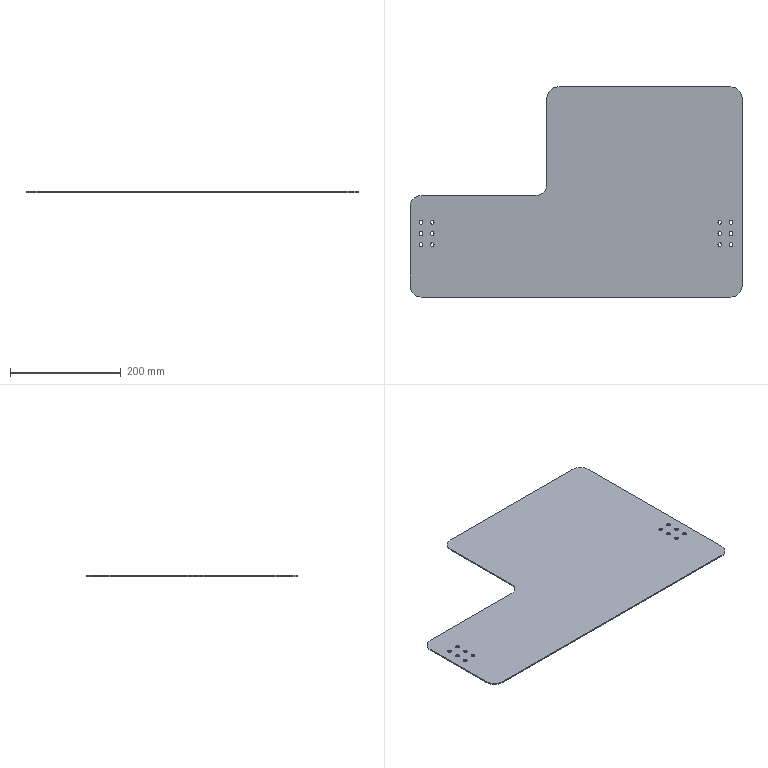Part | STEP file | MT-COMBO-119-S010 | 1 solid | 38 faces | box 600 x 380 x 2 mm | volume 357256 mm3 | cylinder 30 | plane 8 | commonest cylinder face diameters 6.8 x24 40 x6
STEP:
#1=CARTESIAN_POINT('',(-263.4,-15.,2.));
#2=VERTEX_POINT('',#1);
#3=CARTESIAN_POINT('',(-256.6,-15.,2.));
#4=VERTEX_POINT('',#3);
#5=CARTESIAN_POINT('',(-260.,-15.,2.));
#6=DIRECTION('',(0.,0.,1.));
#7=DIRECTION('',(1.,0.,0.));
#8=AXIS2_PLACEMENT_3D('',#5,#6,#7);
#9=CIRCLE('',#8,3.4);
#10=EDGE_CURVE('',#2,#4,#9,.T.);
#11=ORIENTED_EDGE('',*,*,#10,.T.);
#12=CARTESIAN_POINT('',(-256.6,-15.,0.));
#13=VERTEX_POINT('',#12);
#14=CARTESIAN_POINT('',(-256.6,-15.,0.));
#15=DIRECTION('',(0.,0.,-1.));
#16=VECTOR('',#15,1000.);
#17=LINE('',#14,#16);
#18=EDGE_CURVE('',#4,#13,#17,.T.);
#19=ORIENTED_EDGE('',*,*,#18,.T.);
#20=CARTESIAN_POINT('',(-263.4,-15.,0.));
#21=VERTEX_POINT('',#20);
#22=CARTESIAN_POINT('',(-260.,-15.,0.));
#23=DIRECTION('',(0.,0.,-1.));
#24=DIRECTION('',(-1.,0.,0.));
#25=AXIS2_PLACEMENT_3D('',#22,#23,#24);
#26=CIRCLE('',#25,3.4);
#27=EDGE_CURVE('',#13,#21,#26,.T.);
#28=ORIENTED_EDGE('',*,*,#27,.T.);
#29=CARTESIAN_POINT('',(-263.4,-15.,0.));
#30=DIRECTION('',(0.,0.,-1.));
#31=VECTOR('',#30,1000.);
#32=LINE('',#29,#31);
#33=EDGE_CURVE('',#2,#21,#32,.T.);
#34=ORIENTED_EDGE('',*,*,#33,.F.);
#35=EDGE_LOOP('',(#11,#19,#28,#34));
#36=FACE_OUTER_BOUND('',#35,.T.);
#37=CARTESIAN_POINT('',(-260.,-15.,0.));
#38=DIRECTION('',(0.,0.,-1.));
#39=DIRECTION('',(-1.,0.,0.));
#40=AXIS2_PLACEMENT_3D('',#37,#38,#39);
#41=CYLINDRICAL_SURFACE('',#40,3.4);
#42=ADVANCED_FACE('',(#36),#41,.F.);
#43=CARTESIAN_POINT('',(-283.4,-15.,2.));
#44=VERTEX_POINT('',#43);
#45=CARTESIAN_POINT('',(-276.6,-15.,2.));
#46=VERTEX_POINT('',#45);
#47=CARTESIAN_POINT('',(-280.,-15.,2.));
#48=DIRECTION('',(0.,0.,1.));
#49=DIRECTION('',(1.,0.,0.));
#50=AXIS2_PLACEMENT_3D('',#47,#48,#49);
#51=CIRCLE('',#50,3.4);
#52=EDGE_CURVE('',#44,#46,#51,.T.);
#53=ORIENTED_EDGE('',*,*,#52,.T.);
#54=CARTESIAN_POINT('',(-276.6,-15.,0.));
#55=VERTEX_POINT('',#54);
#56=CARTESIAN_POINT('',(-276.6,-15.,0.));
#57=DIRECTION('',(0.,0.,-1.));
#58=VECTOR('',#57,1000.);
#59=LINE('',#56,#58);
#60=EDGE_CURVE('',#46,#55,#59,.T.);
#61=ORIENTED_EDGE('',*,*,#60,.T.);
#62=CARTESIAN_POINT('',(-283.4,-15.,0.));
#63=VERTEX_POINT('',#62);
#64=CARTESIAN_POINT('',(-280.,-15.,0.));
#65=DIRECTION('',(0.,0.,-1.));
#66=DIRECTION('',(-1.,0.,0.));
#67=AXIS2_PLACEMENT_3D('',#64,#65,#66);
#68=CIRCLE('',#67,3.4);
#69=EDGE_CURVE('',#55,#63,#68,.T.);
#70=ORIENTED_EDGE('',*,*,#69,.T.);
#71=CARTESIAN_POINT('',(-283.4,-15.,0.));
#72=DIRECTION('',(0.,0.,-1.));
#73=VECTOR('',#72,1000.);
#74=LINE('',#71,#73);
#75=EDGE_CURVE('',#44,#63,#74,.T.);
#76=ORIENTED_EDGE('',*,*,#75,.F.);
#77=EDGE_LOOP('',(#53,#61,#70,#76));
#78=FACE_OUTER_BOUND('',#77,.T.);
#79=CARTESIAN_POINT('',(-280.,-15.,0.));
#80=DIRECTION('',(0.,0.,-1.));
#81=DIRECTION('',(-1.,0.,0.));
#82=AXIS2_PLACEMENT_3D('',#79,#80,#81);
#83=CYLINDRICAL_SURFACE('',#82,3.4);
#84=ADVANCED_FACE('',(#78),#83,.F.);
#85=CARTESIAN_POINT('',(-263.4,-35.,2.));
#86=VERTEX_POINT('',#85);
#87=CARTESIAN_POINT('',(-256.6,-35.,2.));
#88=VERTEX_POINT('',#87);
#89=CARTESIAN_POINT('',(-260.,-35.,2.));
#90=DIRECTION('',(0.,0.,1.));
#91=DIRECTION('',(1.,0.,0.));
#92=AXIS2_PLACEMENT_3D('',#89,#90,#91);
#93=CIRCLE('',#92,3.4);
#94=EDGE_CURVE('',#86,#88,#93,.T.);
#95=ORIENTED_EDGE('',*,*,#94,.T.);
#96=CARTESIAN_POINT('',(-256.6,-35.,0.));
#97=VERTEX_POINT('',#96);
#98=CARTESIAN_POINT('',(-256.6,-35.,0.));
#99=DIRECTION('',(0.,0.,-1.));
#100=VECTOR('',#99,1000.);
#101=LINE('',#98,#100);
#102=EDGE_CURVE('',#88,#97,#101,.T.);
#103=ORIENTED_EDGE('',*,*,#102,.T.);
#104=CARTESIAN_POINT('',(-263.4,-35.,0.));
#105=VERTEX_POINT('',#104);
#106=CARTESIAN_POINT('',(-260.,-35.,0.));
#107=DIRECTION('',(0.,0.,-1.));
#108=DIRECTION('',(-1.,0.,0.));
#109=AXIS2_PLACEMENT_3D('',#106,#107,#108);
#110=CIRCLE('',#109,3.4);
#111=EDGE_CURVE('',#97,#105,#110,.T.);
#112=ORIENTED_EDGE('',*,*,#111,.T.);
#113=CARTESIAN_POINT('',(-263.4,-35.,0.));
#114=DIRECTION('',(0.,0.,-1.));
#115=VECTOR('',#114,1000.);
#116=LINE('',#113,#115);
#117=EDGE_CURVE('',#86,#105,#116,.T.);
#118=ORIENTED_EDGE('',*,*,#117,.F.);
#119=EDGE_LOOP('',(#95,#103,#112,#118));
#120=FACE_OUTER_BOUND('',#119,.T.);
#121=CARTESIAN_POINT('',(-260.,-35.,0.));
#122=DIRECTION('',(0.,0.,-1.));
#123=DIRECTION('',(-1.,0.,0.));
#124=AXIS2_PLACEMENT_3D('',#121,#122,#123);
#125=CYLINDRICAL_SURFACE('',#124,3.4);
#126=ADVANCED_FACE('',(#120),#125,.F.);
#127=CARTESIAN_POINT('',(-283.4,-35.,2.));
#128=VERTEX_POINT('',#127);
#129=CARTESIAN_POINT('',(-276.6,-35.,2.));
#130=VERTEX_POINT('',#129);
#131=CARTESIAN_POINT('',(-280.,-35.,2.));
#132=DIRECTION('',(0.,0.,1.));
#133=DIRECTION('',(1.,0.,0.));
#134=AXIS2_PLACEMENT_3D('',#131,#132,#133);
#135=CIRCLE('',#134,3.4);
#136=EDGE_CURVE('',#128,#130,#135,.T.);
#137=ORIENTED_EDGE('',*,*,#136,.T.);
#138=CARTESIAN_POINT('',(-276.6,-35.,0.));
#139=VERTEX_POINT('',#138);
#140=CARTESIAN_POINT('',(-276.6,-35.,0.));
#141=DIRECTION('',(0.,0.,-1.));
#142=VECTOR('',#141,1000.);
#143=LINE('',#140,#142);
#144=EDGE_CURVE('',#130,#139,#143,.T.);
#145=ORIENTED_EDGE('',*,*,#144,.T.);
#146=CARTESIAN_POINT('',(-283.4,-35.,0.));
#147=VERTEX_POINT('',#146);
#148=CARTESIAN_POINT('',(-280.,-35.,0.));
#149=DIRECTION('',(0.,0.,-1.));
#150=DIRECTION('',(-1.,0.,0.));
#151=AXIS2_PLACEMENT_3D('',#148,#149,#150);
#152=CIRCLE('',#151,3.4);
#153=EDGE_CURVE('',#139,#147,#152,.T.);
#154=ORIENTED_EDGE('',*,*,#153,.T.);
#155=CARTESIAN_POINT('',(-283.4,-35.,0.));
#156=DIRECTION('',(0.,0.,-1.));
#157=VECTOR('',#156,1000.);
#158=LINE('',#155,#157);
#159=EDGE_CURVE('',#128,#147,#158,.T.);
#160=ORIENTED_EDGE('',*,*,#159,.F.);
#161=EDGE_LOOP('',(#137,#145,#154,#160));
#162=FACE_OUTER_BOUND('',#161,.T.);
#163=CARTESIAN_POINT('',(-280.,-35.,0.));
#164=DIRECTION('',(0.,0.,-1.));
#165=DIRECTION('',(-1.,0.,0.));
#166=AXIS2_PLACEMENT_3D('',#163,#164,#165);
#167=CYLINDRICAL_SURFACE('',#166,3.4);
#168=ADVANCED_FACE('',(#162),#167,.F.);
#169=CARTESIAN_POINT('',(-283.4,-55.,2.));
#170=VERTEX_POINT('',#169);
#171=CARTESIAN_POINT('',(-276.6,-55.,2.));
#172=VERTEX_POINT('',#171);
#173=CARTESIAN_POINT('',(-280.,-55.,2.));
#174=DIRECTION('',(0.,0.,1.));
#175=DIRECTION('',(1.,0.,0.));
#176=AXIS2_PLACEMENT_3D('',#173,#174,#175);
#177=CIRCLE('',#176,3.4);
#178=EDGE_CURVE('',#170,#172,#177,.T.);
#179=ORIENTED_EDGE('',*,*,#178,.T.);
#180=CARTESIAN_POINT('',(-276.6,-55.,0.));
#181=VERTEX_POINT('',#180);
#182=CARTESIAN_POINT('',(-276.6,-55.,0.));
#183=DIRECTION('',(0.,0.,-1.));
#184=VECTOR('',#183,1000.);
#185=LINE('',#182,#184);
#186=EDGE_CURVE('',#172,#181,#185,.T.);
#187=ORIENTED_EDGE('',*,*,#186,.T.);
#188=CARTESIAN_POINT('',(-283.4,-55.,0.));
#189=VERTEX_POINT('',#188);
#190=CARTESIAN_POINT('',(-280.,-55.,0.));
#191=DIRECTION('',(0.,0.,-1.));
#192=DIRECTION('',(-1.,0.,0.));
#193=AXIS2_PLACEMENT_3D('',#190,#191,#192);
#194=CIRCLE('',#193,3.4);
#195=EDGE_CURVE('',#181,#189,#194,.T.);
#196=ORIENTED_EDGE('',*,*,#195,.T.);
#197=CARTESIAN_POINT('',(-283.4,-55.,0.));
#198=DIRECTION('',(0.,0.,-1.));
#199=VECTOR('',#198,1000.);
#200=LINE('',#197,#199);
#201=EDGE_CURVE('',#170,#189,#200,.T.);
#202=ORIENTED_EDGE('',*,*,#201,.F.);
#203=EDGE_LOOP('',(#179,#187,#196,#202));
#204=FACE_OUTER_BOUND('',#203,.T.);
#205=CARTESIAN_POINT('',(-280.,-55.,0.));
#206=DIRECTION('',(0.,0.,-1.));
#207=DIRECTION('',(-1.,0.,0.));
#208=AXIS2_PLACEMENT_3D('',#205,#206,#207);
#209=CYLINDRICAL_SURFACE('',#208,3.4);
#210=ADVANCED_FACE('',(#204),#209,.F.);
#211=CARTESIAN_POINT('',(-263.4,-55.,2.));
#212=VERTEX_POINT('',#211);
#213=CARTESIAN_POINT('',(-256.6,-55.,2.));
#214=VERTEX_POINT('',#213);
#215=CARTESIAN_POINT('',(-260.,-55.,2.));
#216=DIRECTION('',(0.,0.,1.));
#217=DIRECTION('',(1.,0.,0.));
#218=AXIS2_PLACEMENT_3D('',#215,#216,#217);
#219=CIRCLE('',#218,3.4);
#220=EDGE_CURVE('',#212,#214,#219,.T.);
#221=ORIENTED_EDGE('',*,*,#220,.T.);
#222=CARTESIAN_POINT('',(-256.6,-55.,0.));
#223=VERTEX_POINT('',#222);
#224=CARTESIAN_POINT('',(-256.6,-55.,0.));
#225=DIRECTION('',(0.,0.,-1.));
#226=VECTOR('',#225,1000.);
#227=LINE('',#224,#226);
#228=EDGE_CURVE('',#214,#223,#227,.T.);
#229=ORIENTED_EDGE('',*,*,#228,.T.);
#230=CARTESIAN_POINT('',(-263.4,-55.,0.));
#231=VERTEX_POINT('',#230);
#232=CARTESIAN_POINT('',(-260.,-55.,0.));
#233=DIRECTION('',(0.,0.,-1.));
#234=DIRECTION('',(-1.,0.,0.));
#235=AXIS2_PLACEMENT_3D('',#232,#233,#234);
#236=CIRCLE('',#235,3.4);
#237=EDGE_CURVE('',#223,#231,#236,.T.);
#238=ORIENTED_EDGE('',*,*,#237,.T.);
#239=CARTESIAN_POINT('',(-263.4,-55.,0.));
#240=DIRECTION('',(0.,0.,-1.));
#241=VECTOR('',#240,1000.);
#242=LINE('',#239,#241);
#243=EDGE_CURVE('',#212,#231,#242,.T.);
#244=ORIENTED_EDGE('',*,*,#243,.F.);
#245=EDGE_LOOP('',(#221,#229,#238,#244));
#246=FACE_OUTER_BOUND('',#245,.T.);
#247=CARTESIAN_POINT('',(-260.,-55.,0.));
#248=DIRECTION('',(0.,0.,-1.));
#249=DIRECTION('',(-1.,0.,0.));
#250=AXIS2_PLACEMENT_3D('',#247,#248,#249);
#251=CYLINDRICAL_SURFACE('',#250,3.4);
#252=ADVANCED_FACE('',(#246),#251,.F.);
#253=CARTESIAN_POINT('',(256.6,-15.,2.));
#254=VERTEX_POINT('',#253);
#255=CARTESIAN_POINT('',(263.4,-15.,2.));
#256=VERTEX_POINT('',#255);
#257=CARTESIAN_POINT('',(260.,-15.,2.));
#258=DIRECTION('',(0.,0.,1.));
#259=DIRECTION('',(1.,0.,0.));
#260=AXIS2_PLACEMENT_3D('',#257,#258,#259);
#261=CIRCLE('',#260,3.4);
#262=EDGE_CURVE('',#254,#256,#261,.T.);
#263=ORIENTED_EDGE('',*,*,#262,.T.);
#264=CARTESIAN_POINT('',(263.4,-15.,0.));
#265=VERTEX_POINT('',#264);
#266=CARTESIAN_POINT('',(263.4,-15.,0.));
#267=DIRECTION('',(0.,0.,-1.));
#268=VECTOR('',#267,1000.);
#269=LINE('',#266,#268);
#270=EDGE_CURVE('',#256,#265,#269,.T.);
#271=ORIENTED_EDGE('',*,*,#270,.T.);
#272=CARTESIAN_POINT('',(256.6,-15.,0.));
#273=VERTEX_POINT('',#272);
#274=CARTESIAN_POINT('',(260.,-15.,0.));
#275=DIRECTION('',(0.,0.,-1.));
#276=DIRECTION('',(-1.,0.,0.));
#277=AXIS2_PLACEMENT_3D('',#274,#275,#276);
#278=CIRCLE('',#277,3.4);
#279=EDGE_CURVE('',#265,#273,#278,.T.);
#280=ORIENTED_EDGE('',*,*,#279,.T.);
#281=CARTESIAN_POINT('',(256.6,-15.,0.));
#282=DIRECTION('',(0.,0.,-1.));
#283=VECTOR('',#282,1000.);
#284=LINE('',#281,#283);
#285=EDGE_CURVE('',#254,#273,#284,.T.);
#286=ORIENTED_EDGE('',*,*,#285,.F.);
#287=EDGE_LOOP('',(#263,#271,#280,#286));
#288=FACE_OUTER_BOUND('',#287,.T.);
#289=CARTESIAN_POINT('',(260.,-15.,0.));
#290=DIRECTION('',(0.,0.,-1.));
#291=DIRECTION('',(-1.,0.,0.));
#292=AXIS2_PLACEMENT_3D('',#289,#290,#291);
#293=CYLINDRICAL_SURFACE('',#292,3.4);
#294=ADVANCED_FACE('',(#288),#293,.F.);
#295=CARTESIAN_POINT('',(276.6,-15.,2.));
#296=VERTEX_POINT('',#295);
#297=CARTESIAN_POINT('',(283.4,-15.,2.));
#298=VERTEX_POINT('',#297);
#299=CARTESIAN_POINT('',(280.,-15.,2.));
#300=DIRECTION('',(0.,0.,1.));
#301=DIRECTION('',(1.,0.,0.));
#302=AXIS2_PLACEMENT_3D('',#299,#300,#301);
#303=CIRCLE('',#302,3.4);
#304=EDGE_CURVE('',#296,#298,#303,.T.);
#305=ORIENTED_EDGE('',*,*,#304,.T.);
#306=CARTESIAN_POINT('',(283.4,-15.,0.));
#307=VERTEX_POINT('',#306);
#308=CARTESIAN_POINT('',(283.4,-15.,0.));
#309=DIRECTION('',(0.,0.,-1.));
#310=VECTOR('',#309,1000.);
#311=LINE('',#308,#310);
#312=EDGE_CURVE('',#298,#307,#311,.T.);
#313=ORIENTED_EDGE('',*,*,#312,.T.);
#314=CARTESIAN_POINT('',(276.6,-15.,0.));
#315=VERTEX_POINT('',#314);
#316=CARTESIAN_POINT('',(280.,-15.,0.));
#317=DIRECTION('',(0.,0.,-1.));
#318=DIRECTION('',(-1.,0.,0.));
#319=AXIS2_PLACEMENT_3D('',#316,#317,#318);
#320=CIRCLE('',#319,3.4);
#321=EDGE_CURVE('',#307,#315,#320,.T.);
#322=ORIENTED_EDGE('',*,*,#321,.T.);
#323=CARTESIAN_POINT('',(276.6,-15.,0.));
#324=DIRECTION('',(0.,0.,-1.));
#325=VECTOR('',#324,1000.);
#326=LINE('',#323,#325);
#327=EDGE_CURVE('',#296,#315,#326,.T.);
#328=ORIENTED_EDGE('',*,*,#327,.F.);
#329=EDGE_LOOP('',(#305,#313,#322,#328));
#330=FACE_OUTER_BOUND('',#329,.T.);
#331=CARTESIAN_POINT('',(280.,-15.,0.));
#332=DIRECTION('',(0.,0.,-1.));
#333=DIRECTION('',(-1.,0.,0.));
#334=AXIS2_PLACEMENT_3D('',#331,#332,#333);
#335=CYLINDRICAL_SURFACE('',#334,3.4);
#336=ADVANCED_FACE('',(#330),#335,.F.);
#337=CARTESIAN_POINT('',(256.6,-35.,2.));
#338=VERTEX_POINT('',#337);
#339=CARTESIAN_POINT('',(263.4,-35.,2.));
#340=VERTEX_POINT('',#339);
#341=CARTESIAN_POINT('',(260.,-35.,2.));
#342=DIRECTION('',(0.,0.,1.));
#343=DIRECTION('',(1.,0.,0.));
#344=AXIS2_PLACEMENT_3D('',#341,#342,#343);
#345=CIRCLE('',#344,3.4);
#346=EDGE_CURVE('',#338,#340,#345,.T.);
#347=ORIENTED_EDGE('',*,*,#346,.T.);
#348=CARTESIAN_POINT('',(263.4,-35.,0.));
#349=VERTEX_POINT('',#348);
#350=CARTESIAN_POINT('',(263.4,-35.,0.));
#351=DIRECTION('',(0.,0.,-1.));
#352=VECTOR('',#351,1000.);
#353=LINE('',#350,#352);
#354=EDGE_CURVE('',#340,#349,#353,.T.);
#355=ORIENTED_EDGE('',*,*,#354,.T.);
#356=CARTESIAN_POINT('',(256.6,-35.,0.));
#357=VERTEX_POINT('',#356);
#358=CARTESIAN_POINT('',(260.,-35.,0.));
#359=DIRECTION('',(0.,0.,-1.));
#360=DIRECTION('',(-1.,0.,0.));
#361=AXIS2_PLACEMENT_3D('',#358,#359,#360);
#362=CIRCLE('',#361,3.4);
#363=EDGE_CURVE('',#349,#357,#362,.T.);
#364=ORIENTED_EDGE('',*,*,#363,.T.);
#365=CARTESIAN_POINT('',(256.6,-35.,0.));
#366=DIRECTION('',(0.,0.,-1.));
#367=VECTOR('',#366,1000.);
#368=LINE('',#365,#367);
#369=EDGE_CURVE('',#338,#357,#368,.T.);
#370=ORIENTED_EDGE('',*,*,#369,.F.);
#371=EDGE_LOOP('',(#347,#355,#364,#370));
#372=FACE_OUTER_BOUND('',#371,.T.);
#373=CARTESIAN_POINT('',(260.,-35.,0.));
#374=DIRECTION('',(0.,0.,-1.));
#375=DIRECTION('',(-1.,0.,0.));
#376=AXIS2_PLACEMENT_3D('',#373,#374,#375);
#377=CYLINDRICAL_SURFACE('',#376,3.4);
#378=ADVANCED_FACE('',(#372),#377,.F.);
#379=CARTESIAN_POINT('',(276.6,-35.,2.));
#380=VERTEX_POINT('',#379);
#381=CARTESIAN_POINT('',(283.4,-35.,2.));
#382=VERTEX_POINT('',#381);
#383=CARTESIAN_POINT('',(280.,-35.,2.));
#384=DIRECTION('',(0.,0.,1.));
#385=DIRECTION('',(1.,0.,0.));
#386=AXIS2_PLACEMENT_3D('',#383,#384,#385);
#387=CIRCLE('',#386,3.4);
#388=EDGE_CURVE('',#380,#382,#387,.T.);
#389=ORIENTED_EDGE('',*,*,#388,.T.);
#390=CARTESIAN_POINT('',(283.4,-35.,0.));
#391=VERTEX_POINT('',#390);
#392=CARTESIAN_POINT('',(283.4,-35.,0.));
#393=DIRECTION('',(0.,0.,-1.));
#394=VECTOR('',#393,1000.);
#395=LINE('',#392,#394);
#396=EDGE_CURVE('',#382,#391,#395,.T.);
#397=ORIENTED_EDGE('',*,*,#396,.T.);
#398=CARTESIAN_POINT('',(276.6,-35.,0.));
#399=VERTEX_POINT('',#398);
#400=CARTESIAN_POINT('',(280.,-35.,0.));
#401=DIRECTION('',(0.,0.,-1.));
#402=DIRECTION('',(-1.,0.,0.));
#403=AXIS2_PLACEMENT_3D('',#400,#401,#402);
#404=CIRCLE('',#403,3.4);
#405=EDGE_CURVE('',#391,#399,#404,.T.);
#406=ORIENTED_EDGE('',*,*,#405,.T.);
#407=CARTESIAN_POINT('',(276.6,-35.,0.));
#408=DIRECTION('',(0.,0.,-1.));
#409=VECTOR('',#408,1000.);
#410=LINE('',#407,#409);
#411=EDGE_CURVE('',#380,#399,#410,.T.);
#412=ORIENTED_EDGE('',*,*,#411,.F.);
#413=EDGE_LOOP('',(#389,#397,#406,#412));
#414=FACE_OUTER_BOUND('',#413,.T.);
#415=CARTESIAN_POINT('',(280.,-35.,0.));
#416=DIRECTION('',(0.,0.,-1.));
#417=DIRECTION('',(-1.,0.,0.));
#418=AXIS2_PLACEMENT_3D('',#415,#416,#417);
#419=CYLINDRICAL_SURFACE('',#418,3.4);
#420=ADVANCED_FACE('',(#414),#419,.F.);
#421=CARTESIAN_POINT('',(276.6,-55.,2.));
#422=VERTEX_POINT('',#421);
#423=CARTESIAN_POINT('',(283.4,-55.,2.));
#424=VERTEX_POINT('',#423);
#425=CARTESIAN_POINT('',(280.,-55.,2.));
#426=DIRECTION('',(0.,0.,1.));
#427=DIRECTION('',(1.,0.,0.));
#428=AXIS2_PLACEMENT_3D('',#425,#426,#427);
#429=CIRCLE('',#428,3.4);
#430=EDGE_CURVE('',#422,#424,#429,.T.);
#431=ORIENTED_EDGE('',*,*,#430,.T.);
#432=CARTESIAN_POINT('',(283.4,-55.,0.));
#433=VERTEX_POINT('',#432);
#434=CARTESIAN_POINT('',(283.4,-55.,0.));
#435=DIRECTION('',(0.,0.,-1.));
#436=VECTOR('',#435,1000.);
#437=LINE('',#434,#436);
#438=EDGE_CURVE('',#424,#433,#437,.T.);
#439=ORIENTED_EDGE('',*,*,#438,.T.);
#440=CARTESIAN_POINT('',(276.6,-55.,0.));
#441=VERTEX_POINT('',#440);
#442=CARTESIAN_POINT('',(280.,-55.,0.));
#443=DIRECTION('',(0.,0.,-1.));
#444=DIRECTION('',(-1.,0.,0.));
#445=AXIS2_PLACEMENT_3D('',#442,#443,#444);
#446=CIRCLE('',#445,3.4);
#447=EDGE_CURVE('',#433,#441,#446,.T.);
#448=ORIENTED_EDGE('',*,*,#447,.T.);
#449=CARTESIAN_POINT('',(276.6,-55.,0.));
#450=DIRECTION('',(0.,0.,-1.));
#451=VECTOR('',#450,1000.);
#452=LINE('',#449,#451);
#453=EDGE_CURVE('',#422,#441,#452,.T.);
#454=ORIENTED_EDGE('',*,*,#453,.F.);
#455=EDGE_LOOP('',(#431,#439,#448,#454));
#456=FACE_OUTER_BOUND('',#455,.T.);
#457=CARTESIAN_POINT('',(280.,-55.,0.));
#458=DIRECTION('',(0.,0.,-1.));
#459=DIRECTION('',(-1.,0.,0.));
#460=AXIS2_PLACEMENT_3D('',#457,#458,#459);
#461=CYLINDRICAL_SURFACE('',#460,3.4);
#462=ADVANCED_FACE('',(#456),#461,.F.);
#463=CARTESIAN_POINT('',(256.6,-55.,2.));
#464=VERTEX_POINT('',#463);
#465=CARTESIAN_POINT('',(263.4,-55.,2.));
#466=VERTEX_POINT('',#465);
#467=CARTESIAN_POINT('',(260.,-55.,2.));
#468=DIRECTION('',(0.,0.,1.));
#469=DIRECTION('',(1.,0.,0.));
#470=AXIS2_PLACEMENT_3D('',#467,#468,#469);
#471=CIRCLE('',#470,3.4);
#472=EDGE_CURVE('',#464,#466,#471,.T.);
#473=ORIENTED_EDGE('',*,*,#472,.T.);
#474=CARTESIAN_POINT('',(263.4,-55.,0.));
#475=VERTEX_POINT('',#474);
#476=CARTESIAN_POINT('',(263.4,-55.,0.));
#477=DIRECTION('',(0.,0.,-1.));
#478=VECTOR('',#477,1000.);
#479=LINE('',#476,#478);
#480=EDGE_CURVE('',#466,#475,#479,.T.);
#481=ORIENTED_EDGE('',*,*,#480,.T.);
#482=CARTESIAN_POINT('',(256.6,-55.,0.));
#483=VERTEX_POINT('',#482);
#484=CARTESIAN_POINT('',(260.,-55.,0.));
#485=DIRECTION('',(0.,0.,-1.));
#486=DIRECTION('',(-1.,0.,0.));
#487=AXIS2_PLACEMENT_3D('',#484,#485,#486);
#488=CIRCLE('',#487,3.4);
#489=EDGE_CURVE('',#475,#483,#488,.T.);
#490=ORIENTED_EDGE('',*,*,#489,.T.);
#491=CARTESIAN_POINT('',(256.6,-55.,0.));
#492=DIRECTION('',(0.,0.,-1.));
#493=VECTOR('',#492,1000.);
#494=LINE('',#491,#493);
#495=EDGE_CURVE('',#464,#483,#494,.T.);
#496=ORIENTED_EDGE('',*,*,#495,.F.);
#497=EDGE_LOOP('',(#473,#481,#490,#496));
#498=FACE_OUTER_BOUND('',#497,.T.);
#499=CARTESIAN_POINT('',(260.,-55.,0.));
#500=DIRECTION('',(0.,0.,-1.));
#501=DIRECTION('',(-1.,0.,0.));
#502=AXIS2_PLACEMENT_3D('',#499,#500,#501);
#503=CYLINDRICAL_SURFACE('',#502,3.4);
#504=ADVANCED_FACE('',(#498),#503,.F.);
#505=CARTESIAN_POINT('',(-260.,-15.,0.));
#506=DIRECTION('',(0.,0.,-1.));
#507=DIRECTION('',(-1.,0.,0.));
#508=AXIS2_PLACEMENT_3D('',#505,#506,#507);
#509=CIRCLE('',#508,3.4);
#510=EDGE_CURVE('',#21,#13,#509,.T.);
#511=ORIENTED_EDGE('',*,*,#510,.F.);
#512=ORIENTED_EDGE('',*,*,#27,.F.);
#513=EDGE_LOOP('',(#511,#512));
#514=FACE_BOUND('',#513,.T.);
#515=CARTESIAN_POINT('',(-280.,-15.,0.));
#516=DIRECTION('',(0.,0.,-1.));
#517=DIRECTION('',(-1.,0.,0.));
#518=AXIS2_PLACEMENT_3D('',#515,#516,#517);
#519=CIRCLE('',#518,3.4);
#520=EDGE_CURVE('',#63,#55,#519,.T.);
#521=ORIENTED_EDGE('',*,*,#520,.F.);
#522=ORIENTED_EDGE('',*,*,#69,.F.);
#523=EDGE_LOOP('',(#521,#522));
#524=FACE_BOUND('',#523,.T.);
#525=CARTESIAN_POINT('',(-260.,-35.,0.));
#526=DIRECTION('',(0.,0.,-1.));
#527=DIRECTION('',(-1.,0.,0.));
#528=AXIS2_PLACEMENT_3D('',#525,#526,#527);
#529=CIRCLE('',#528,3.4);
#530=EDGE_CURVE('',#105,#97,#529,.T.);
#531=ORIENTED_EDGE('',*,*,#530,.F.);
#532=ORIENTED_EDGE('',*,*,#111,.F.);
#533=EDGE_LOOP('',(#531,#532));
#534=FACE_BOUND('',#533,.T.);
#535=CARTESIAN_POINT('',(-280.,-35.,0.));
#536=DIRECTION('',(0.,0.,-1.));
#537=DIRECTION('',(-1.,0.,0.));
#538=AXIS2_PLACEMENT_3D('',#535,#536,#537);
#539=CIRCLE('',#538,3.4);
#540=EDGE_CURVE('',#147,#139,#539,.T.);
#541=ORIENTED_EDGE('',*,*,#540,.F.);
#542=ORIENTED_EDGE('',*,*,#153,.F.);
#543=EDGE_LOOP('',(#541,#542));
#544=FACE_BOUND('',#543,.T.);
#545=CARTESIAN_POINT('',(-280.,-55.,0.));
#546=DIRECTION('',(0.,0.,-1.));
#547=DIRECTION('',(-1.,0.,0.));
#548=AXIS2_PLACEMENT_3D('',#545,#546,#547);
#549=CIRCLE('',#548,3.4);
#550=EDGE_CURVE('',#189,#181,#549,.T.);
#551=ORIENTED_EDGE('',*,*,#550,.F.);
#552=ORIENTED_EDGE('',*,*,#195,.F.);
#553=EDGE_LOOP('',(#551,#552));
#554=FACE_BOUND('',#553,.T.);
#555=CARTESIAN_POINT('',(260.,-15.,0.));
#556=DIRECTION('',(0.,0.,-1.));
#557=DIRECTION('',(-1.,0.,0.));
#558=AXIS2_PLACEMENT_3D('',#555,#556,#557);
#559=CIRCLE('',#558,3.4);
#560=EDGE_CURVE('',#273,#265,#559,.T.);
#561=ORIENTED_EDGE('',*,*,#560,.F.);
#562=ORIENTED_EDGE('',*,*,#279,.F.);
#563=EDGE_LOOP('',(#561,#562));
#564=FACE_BOUND('',#563,.T.);
#565=CARTESIAN_POINT('',(280.,-15.,0.));
#566=DIRECTION('',(0.,0.,-1.));
#567=DIRECTION('',(-1.,0.,0.));
#568=AXIS2_PLACEMENT_3D('',#565,#566,#567);
#569=CIRCLE('',#568,3.4);
#570=EDGE_CURVE('',#315,#307,#569,.T.);
#571=ORIENTED_EDGE('',*,*,#570,.F.);
#572=ORIENTED_EDGE('',*,*,#321,.F.);
#573=EDGE_LOOP('',(#571,#572));
#574=FACE_BOUND('',#573,.T.);
#575=CARTESIAN_POINT('',(260.,-35.,0.));
#576=DIRECTION('',(0.,0.,-1.));
#577=DIRECTION('',(-1.,0.,0.));
#578=AXIS2_PLACEMENT_3D('',#575,#576,#577);
#579=CIRCLE('',#578,3.4);
#580=EDGE_CURVE('',#357,#349,#579,.T.);
#581=ORIENTED_EDGE('',*,*,#580,.F.);
#582=ORIENTED_EDGE('',*,*,#363,.F.);
#583=EDGE_LOOP('',(#581,#582));
#584=FACE_BOUND('',#583,.T.);
#585=CARTESIAN_POINT('',(280.,-35.,0.));
#586=DIRECTION('',(0.,0.,-1.));
#587=DIRECTION('',(-1.,0.,0.));
#588=AXIS2_PLACEMENT_3D('',#585,#586,#587);
#589=CIRCLE('',#588,3.4);
#590=EDGE_CURVE('',#399,#391,#589,.T.);
#591=ORIENTED_EDGE('',*,*,#590,.F.);
#592=ORIENTED_EDGE('',*,*,#405,.F.);
#593=EDGE_LOOP('',(#591,#592));
#594=FACE_BOUND('',#593,.T.);
#595=CARTESIAN_POINT('',(280.,-55.,0.));
#596=DIRECTION('',(0.,0.,-1.));
#597=DIRECTION('',(-1.,0.,0.));
#598=AXIS2_PLACEMENT_3D('',#595,#596,#597);
#599=CIRCLE('',#598,3.4);
#600=EDGE_CURVE('',#441,#433,#599,.T.);
#601=ORIENTED_EDGE('',*,*,#600,.F.);
#602=ORIENTED_EDGE('',*,*,#447,.F.);
#603=EDGE_LOOP('',(#601,#602));
#604=FACE_BOUND('',#603,.T.);
#605=CARTESIAN_POINT('',(260.,-55.,0.));
#606=DIRECTION('',(0.,0.,-1.));
#607=DIRECTION('',(-1.,0.,0.));
#608=AXIS2_PLACEMENT_3D('',#605,#606,#607);
#609=CIRCLE('',#608,3.4);
#610=EDGE_CURVE('',#483,#475,#609,.T.);
#611=ORIENTED_EDGE('',*,*,#610,.F.);
#612=ORIENTED_EDGE('',*,*,#489,.F.);
#613=EDGE_LOOP('',(#611,#612));
#614=FACE_BOUND('',#613,.T.);
#615=CARTESIAN_POINT('',(300.,-130.,0.));
#616=VERTEX_POINT('',#615);
#617=CARTESIAN_POINT('',(300.,210.,0.));
#618=VERTEX_POINT('',#617);
#619=CARTESIAN_POINT('',(300.,-150.,0.));
#620=DIRECTION('',(0.,1.,0.));
#621=VECTOR('',#620,1000.);
#622=LINE('',#619,#621);
#623=EDGE_CURVE('',#616,#618,#622,.T.);
#624=ORIENTED_EDGE('',*,*,#623,.F.);
#625=CARTESIAN_POINT('',(280.,-150.,0.));
#626=VERTEX_POINT('',#625);
#627=CARTESIAN_POINT('',(280.,-130.,0.));
#628=DIRECTION('',(0.,0.,-1.));
#629=DIRECTION('',(1.,0.,0.));
#630=AXIS2_PLACEMENT_3D('',#627,#628,#629);
#631=CIRCLE('',#630,20.);
#632=EDGE_CURVE('',#616,#626,#631,.T.);
#633=ORIENTED_EDGE('',*,*,#632,.T.);
#634=CARTESIAN_POINT('',(-280.,-150.,0.));
#635=VERTEX_POINT('',#634);
#636=CARTESIAN_POINT('',(300.,-150.,0.));
#637=DIRECTION('',(1.,0.,0.));
#638=VECTOR('',#637,1000.);
#639=LINE('',#636,#638);
#640=EDGE_CURVE('',#635,#626,#639,.T.);
#641=ORIENTED_EDGE('',*,*,#640,.F.);
#642=CARTESIAN_POINT('',(-300.,-130.,0.));
#643=VERTEX_POINT('',#642);
#644=CARTESIAN_POINT('',(-280.,-130.,0.));
#645=DIRECTION('',(0.,0.,-1.));
#646=DIRECTION('',(1.,0.,0.));
#647=AXIS2_PLACEMENT_3D('',#644,#645,#646);
#648=CIRCLE('',#647,20.);
#649=EDGE_CURVE('',#635,#643,#648,.T.);
#650=ORIENTED_EDGE('',*,*,#649,.T.);
#651=CARTESIAN_POINT('',(-300.,13.637,0.));
#652=VERTEX_POINT('',#651);
#653=CARTESIAN_POINT('',(-300.,-150.,0.));
#654=DIRECTION('',(0.,-1.,0.));
#655=VECTOR('',#654,1000.);
#656=LINE('',#653,#655);
#657=EDGE_CURVE('',#652,#643,#656,.T.);
#658=ORIENTED_EDGE('',*,*,#657,.F.);
#659=CARTESIAN_POINT('',(-280.,33.637,0.));
#660=VERTEX_POINT('',#659);
#661=CARTESIAN_POINT('',(-280.,13.637,0.));
#662=DIRECTION('',(0.,0.,-1.));
#663=DIRECTION('',(1.,0.,0.));
#664=AXIS2_PLACEMENT_3D('',#661,#662,#663);
#665=CIRCLE('',#664,20.);
#666=EDGE_CURVE('',#652,#660,#665,.T.);
#667=ORIENTED_EDGE('',*,*,#666,.T.);
#668=CARTESIAN_POINT('',(-72.537,33.637,0.));
#669=VERTEX_POINT('',#668);
#670=CARTESIAN_POINT('',(-300.,33.637,0.));
#671=DIRECTION('',(-1.,0.,0.));
#672=VECTOR('',#671,1000.);
#673=LINE('',#670,#672);
#674=EDGE_CURVE('',#669,#660,#673,.T.);
#675=ORIENTED_EDGE('',*,*,#674,.F.);
#676=CARTESIAN_POINT('',(-52.537,53.637,0.));
#677=VERTEX_POINT('',#676);
#678=CARTESIAN_POINT('',(-72.537,53.637,0.));
#679=DIRECTION('',(0.,0.,1.));
#680=DIRECTION('',(1.,0.,0.));
#681=AXIS2_PLACEMENT_3D('',#678,#679,#680);
#682=CIRCLE('',#681,20.);
#683=EDGE_CURVE('',#669,#677,#682,.T.);
#684=ORIENTED_EDGE('',*,*,#683,.T.);
#685=CARTESIAN_POINT('',(-52.537,210.,0.));
#686=VERTEX_POINT('',#685);
#687=CARTESIAN_POINT('',(-52.537,150.,0.));
#688=DIRECTION('',(0.,-1.,0.));
#689=VECTOR('',#688,1000.);
#690=LINE('',#687,#689);
#691=EDGE_CURVE('',#686,#677,#690,.T.);
#692=ORIENTED_EDGE('',*,*,#691,.F.);
#693=CARTESIAN_POINT('',(-32.537,230.,0.));
#694=VERTEX_POINT('',#693);
#695=CARTESIAN_POINT('',(-32.537,210.,0.));
#696=DIRECTION('',(0.,0.,-1.));
#697=DIRECTION('',(1.,0.,0.));
#698=AXIS2_PLACEMENT_3D('',#695,#696,#697);
#699=CIRCLE('',#698,20.);
#700=EDGE_CURVE('',#686,#694,#699,.T.);
#701=ORIENTED_EDGE('',*,*,#700,.T.);
#702=CARTESIAN_POINT('',(280.,230.,0.));
#703=VERTEX_POINT('',#702);
#704=CARTESIAN_POINT('',(300.,230.,0.));
#705=DIRECTION('',(-1.,0.,0.));
#706=VECTOR('',#705,1000.);
#707=LINE('',#704,#706);
#708=EDGE_CURVE('',#703,#694,#707,.T.);
#709=ORIENTED_EDGE('',*,*,#708,.F.);
#710=CARTESIAN_POINT('',(280.,210.,0.));
#711=DIRECTION('',(0.,0.,-1.));
#712=DIRECTION('',(1.,0.,0.));
#713=AXIS2_PLACEMENT_3D('',#710,#711,#712);
#714=CIRCLE('',#713,20.);
#715=EDGE_CURVE('',#703,#618,#714,.T.);
#716=ORIENTED_EDGE('',*,*,#715,.T.);
#717=EDGE_LOOP('',(#624,#633,#641,#650,#658,#667,#675,#684,#692,#701,#709,#716));
#718=FACE_OUTER_BOUND('',#717,.T.);
#719=CARTESIAN_POINT('',(-260.,-55.,0.));
#720=DIRECTION('',(0.,0.,-1.));
#721=DIRECTION('',(-1.,0.,0.));
#722=AXIS2_PLACEMENT_3D('',#719,#720,#721);
#723=CIRCLE('',#722,3.4);
#724=EDGE_CURVE('',#231,#223,#723,.T.);
#725=ORIENTED_EDGE('',*,*,#724,.F.);
#726=ORIENTED_EDGE('',*,*,#237,.F.);
#727=EDGE_LOOP('',(#725,#726));
#728=FACE_BOUND('',#727,.T.);
#729=CARTESIAN_POINT('',(0.,0.,0.));
#730=DIRECTION('',(0.,0.,1.));
#731=DIRECTION('',(1.,0.,0.));
#732=AXIS2_PLACEMENT_3D('',#729,#730,#731);
#733=PLANE('',#732);
#734=ADVANCED_FACE('',(#514,#524,#534,#544,#554,#564,#574,#584,#594,#604,#614,#718,#728),#733,.F.);
#735=ORIENTED_EDGE('',*,*,#657,.T.);
#736=CARTESIAN_POINT('',(-300.,-130.,2.));
#737=VERTEX_POINT('',#736);
#738=CARTESIAN_POINT('',(-300.,-130.,2.));
#739=DIRECTION('',(0.,0.,1.));
#740=VECTOR('',#739,1000.);
#741=LINE('',#738,#740);
#742=EDGE_CURVE('',#643,#737,#741,.T.);
#743=ORIENTED_EDGE('',*,*,#742,.T.);
#744=CARTESIAN_POINT('',(-300.,13.637,2.));
#745=VERTEX_POINT('',#744);
#746=CARTESIAN_POINT('',(-300.,-150.,2.));
#747=DIRECTION('',(0.,-1.,0.));
#748=VECTOR('',#747,1000.);
#749=LINE('',#746,#748);
#750=EDGE_CURVE('',#745,#737,#749,.T.);
#751=ORIENTED_EDGE('',*,*,#750,.F.);
#752=CARTESIAN_POINT('',(-300.,13.637,2.));
#753=DIRECTION('',(0.,0.,-1.));
#754=VECTOR('',#753,1000.);
#755=LINE('',#752,#754);
#756=EDGE_CURVE('',#745,#652,#755,.T.);
#757=ORIENTED_EDGE('',*,*,#756,.T.);
#758=EDGE_LOOP('',(#735,#743,#751,#757));
#759=FACE_OUTER_BOUND('',#758,.T.);
#760=CARTESIAN_POINT('',(-300.,-150.,2.));
#761=DIRECTION('',(1.,0.,0.));
#762=DIRECTION('',(0.,0.,-1.));
#763=AXIS2_PLACEMENT_3D('',#760,#761,#762);
#764=PLANE('',#763);
#765=ADVANCED_FACE('',(#759),#764,.F.);
#766=ORIENTED_EDGE('',*,*,#640,.T.);
#767=CARTESIAN_POINT('',(280.,-150.,2.));
#768=VERTEX_POINT('',#767);
#769=CARTESIAN_POINT('',(280.,-150.,2.));
#770=DIRECTION('',(0.,0.,1.));
#771=VECTOR('',#770,1000.);
#772=LINE('',#769,#771);
#773=EDGE_CURVE('',#626,#768,#772,.T.);
#774=ORIENTED_EDGE('',*,*,#773,.T.);
#775=CARTESIAN_POINT('',(-280.,-150.,2.));
#776=VERTEX_POINT('',#775);
#777=CARTESIAN_POINT('',(300.,-150.,2.));
#778=DIRECTION('',(1.,0.,0.));
#779=VECTOR('',#778,1000.);
#780=LINE('',#777,#779);
#781=EDGE_CURVE('',#776,#768,#780,.T.);
#782=ORIENTED_EDGE('',*,*,#781,.F.);
#783=CARTESIAN_POINT('',(-280.,-150.,2.));
#784=DIRECTION('',(0.,0.,-1.));
#785=VECTOR('',#784,1000.);
#786=LINE('',#783,#785);
#787=EDGE_CURVE('',#776,#635,#786,.T.);
#788=ORIENTED_EDGE('',*,*,#787,.T.);
#789=EDGE_LOOP('',(#766,#774,#782,#788));
#790=FACE_OUTER_BOUND('',#789,.T.);
#791=CARTESIAN_POINT('',(300.,-150.,2.));
#792=DIRECTION('',(0.,1.,0.));
#793=DIRECTION('',(0.,0.,1.));
#794=AXIS2_PLACEMENT_3D('',#791,#792,#793);
#795=PLANE('',#794);
#796=ADVANCED_FACE('',(#790),#795,.F.);
#797=CARTESIAN_POINT('',(300.,-130.,2.));
#798=VERTEX_POINT('',#797);
#799=CARTESIAN_POINT('',(300.,210.,2.));
#800=VERTEX_POINT('',#799);
#801=CARTESIAN_POINT('',(300.,-150.,2.));
#802=DIRECTION('',(0.,1.,0.));
#803=VECTOR('',#802,1000.);
#804=LINE('',#801,#803);
#805=EDGE_CURVE('',#798,#800,#804,.T.);
#806=ORIENTED_EDGE('',*,*,#805,.F.);
#807=CARTESIAN_POINT('',(300.,-130.,2.));
#808=DIRECTION('',(0.,0.,-1.));
#809=VECTOR('',#808,1000.);
#810=LINE('',#807,#809);
#811=EDGE_CURVE('',#798,#616,#810,.T.);
#812=ORIENTED_EDGE('',*,*,#811,.T.);
#813=ORIENTED_EDGE('',*,*,#623,.T.);
#814=CARTESIAN_POINT('',(300.,210.,2.));
#815=DIRECTION('',(0.,0.,1.));
#816=VECTOR('',#815,1000.);
#817=LINE('',#814,#816);
#818=EDGE_CURVE('',#618,#800,#817,.T.);
#819=ORIENTED_EDGE('',*,*,#818,.T.);
#820=EDGE_LOOP('',(#806,#812,#813,#819));
#821=FACE_OUTER_BOUND('',#820,.T.);
#822=CARTESIAN_POINT('',(300.,-150.,2.));
#823=DIRECTION('',(-1.,0.,0.));
#824=DIRECTION('',(0.,0.,1.));
#825=AXIS2_PLACEMENT_3D('',#822,#823,#824);
#826=PLANE('',#825);
#827=ADVANCED_FACE('',(#821),#826,.F.);
#828=ORIENTED_EDGE('',*,*,#708,.T.);
#829=CARTESIAN_POINT('',(-32.537,230.,2.));
#830=VERTEX_POINT('',#829);
#831=CARTESIAN_POINT('',(-32.537,230.,2.));
#832=DIRECTION('',(0.,0.,1.));
#833=VECTOR('',#832,1000.);
#834=LINE('',#831,#833);
#835=EDGE_CURVE('',#694,#830,#834,.T.);
#836=ORIENTED_EDGE('',*,*,#835,.T.);
#837=CARTESIAN_POINT('',(280.,230.,2.));
#838=VERTEX_POINT('',#837);
#839=CARTESIAN_POINT('',(300.,230.,2.));
#840=DIRECTION('',(-1.,0.,0.));
#841=VECTOR('',#840,1000.);
#842=LINE('',#839,#841);
#843=EDGE_CURVE('',#838,#830,#842,.T.);
#844=ORIENTED_EDGE('',*,*,#843,.F.);
#845=CARTESIAN_POINT('',(280.,230.,2.));
#846=DIRECTION('',(0.,0.,-1.));
#847=VECTOR('',#846,1000.);
#848=LINE('',#845,#847);
#849=EDGE_CURVE('',#838,#703,#848,.T.);
#850=ORIENTED_EDGE('',*,*,#849,.T.);
#851=EDGE_LOOP('',(#828,#836,#844,#850));
#852=FACE_OUTER_BOUND('',#851,.T.);
#853=CARTESIAN_POINT('',(300.,230.,2.));
#854=DIRECTION('',(0.,-1.,0.));
#855=DIRECTION('',(0.,0.,-1.));
#856=AXIS2_PLACEMENT_3D('',#853,#854,#855);
#857=PLANE('',#856);
#858=ADVANCED_FACE('',(#852),#857,.F.);
#859=ORIENTED_EDGE('',*,*,#10,.F.);
#860=CARTESIAN_POINT('',(-260.,-15.,2.));
#861=DIRECTION('',(0.,0.,1.));
#862=DIRECTION('',(1.,0.,0.));
#863=AXIS2_PLACEMENT_3D('',#860,#861,#862);
#864=CIRCLE('',#863,3.4);
#865=EDGE_CURVE('',#4,#2,#864,.T.);
#866=ORIENTED_EDGE('',*,*,#865,.F.);
#867=EDGE_LOOP('',(#859,#866));
#868=FACE_BOUND('',#867,.T.);
#869=ORIENTED_EDGE('',*,*,#52,.F.);
#870=CARTESIAN_POINT('',(-280.,-15.,2.));
#871=DIRECTION('',(0.,0.,1.));
#872=DIRECTION('',(1.,0.,0.));
#873=AXIS2_PLACEMENT_3D('',#870,#871,#872);
#874=CIRCLE('',#873,3.4);
#875=EDGE_CURVE('',#46,#44,#874,.T.);
#876=ORIENTED_EDGE('',*,*,#875,.F.);
#877=EDGE_LOOP('',(#869,#876));
#878=FACE_BOUND('',#877,.T.);
#879=ORIENTED_EDGE('',*,*,#94,.F.);
#880=CARTESIAN_POINT('',(-260.,-35.,2.));
#881=DIRECTION('',(0.,0.,1.));
#882=DIRECTION('',(1.,0.,0.));
#883=AXIS2_PLACEMENT_3D('',#880,#881,#882);
#884=CIRCLE('',#883,3.4);
#885=EDGE_CURVE('',#88,#86,#884,.T.);
#886=ORIENTED_EDGE('',*,*,#885,.F.);
#887=EDGE_LOOP('',(#879,#886));
#888=FACE_BOUND('',#887,.T.);
#889=ORIENTED_EDGE('',*,*,#136,.F.);
#890=CARTESIAN_POINT('',(-280.,-35.,2.));
#891=DIRECTION('',(0.,0.,1.));
#892=DIRECTION('',(1.,0.,0.));
#893=AXIS2_PLACEMENT_3D('',#890,#891,#892);
#894=CIRCLE('',#893,3.4);
#895=EDGE_CURVE('',#130,#128,#894,.T.);
#896=ORIENTED_EDGE('',*,*,#895,.F.);
#897=EDGE_LOOP('',(#889,#896));
#898=FACE_BOUND('',#897,.T.);
#899=ORIENTED_EDGE('',*,*,#178,.F.);
#900=CARTESIAN_POINT('',(-280.,-55.,2.));
#901=DIRECTION('',(0.,0.,1.));
#902=DIRECTION('',(1.,0.,0.));
#903=AXIS2_PLACEMENT_3D('',#900,#901,#902);
#904=CIRCLE('',#903,3.4);
#905=EDGE_CURVE('',#172,#170,#904,.T.);
#906=ORIENTED_EDGE('',*,*,#905,.F.);
#907=EDGE_LOOP('',(#899,#906));
#908=FACE_BOUND('',#907,.T.);
#909=ORIENTED_EDGE('',*,*,#220,.F.);
#910=CARTESIAN_POINT('',(-260.,-55.,2.));
#911=DIRECTION('',(0.,0.,1.));
#912=DIRECTION('',(1.,0.,0.));
#913=AXIS2_PLACEMENT_3D('',#910,#911,#912);
#914=CIRCLE('',#913,3.4);
#915=EDGE_CURVE('',#214,#212,#914,.T.);
#916=ORIENTED_EDGE('',*,*,#915,.F.);
#917=EDGE_LOOP('',(#909,#916));
#918=FACE_BOUND('',#917,.T.);
#919=ORIENTED_EDGE('',*,*,#262,.F.);
#920=CARTESIAN_POINT('',(260.,-15.,2.));
#921=DIRECTION('',(0.,0.,1.));
#922=DIRECTION('',(1.,0.,0.));
#923=AXIS2_PLACEMENT_3D('',#920,#921,#922);
#924=CIRCLE('',#923,3.4);
#925=EDGE_CURVE('',#256,#254,#924,.T.);
#926=ORIENTED_EDGE('',*,*,#925,.F.);
#927=EDGE_LOOP('',(#919,#926));
#928=FACE_BOUND('',#927,.T.);
#929=ORIENTED_EDGE('',*,*,#304,.F.);
#930=CARTESIAN_POINT('',(280.,-15.,2.));
#931=DIRECTION('',(0.,0.,1.));
#932=DIRECTION('',(1.,0.,0.));
#933=AXIS2_PLACEMENT_3D('',#930,#931,#932);
#934=CIRCLE('',#933,3.4);
#935=EDGE_CURVE('',#298,#296,#934,.T.);
#936=ORIENTED_EDGE('',*,*,#935,.F.);
#937=EDGE_LOOP('',(#929,#936));
#938=FACE_BOUND('',#937,.T.);
#939=ORIENTED_EDGE('',*,*,#346,.F.);
#940=CARTESIAN_POINT('',(260.,-35.,2.));
#941=DIRECTION('',(0.,0.,1.));
#942=DIRECTION('',(1.,0.,0.));
#943=AXIS2_PLACEMENT_3D('',#940,#941,#942);
#944=CIRCLE('',#943,3.4);
#945=EDGE_CURVE('',#340,#338,#944,.T.);
#946=ORIENTED_EDGE('',*,*,#945,.F.);
#947=EDGE_LOOP('',(#939,#946));
#948=FACE_BOUND('',#947,.T.);
#949=ORIENTED_EDGE('',*,*,#388,.F.);
#950=CARTESIAN_POINT('',(280.,-35.,2.));
#951=DIRECTION('',(0.,0.,1.));
#952=DIRECTION('',(1.,0.,0.));
#953=AXIS2_PLACEMENT_3D('',#950,#951,#952);
#954=CIRCLE('',#953,3.4);
#955=EDGE_CURVE('',#382,#380,#954,.T.);
#956=ORIENTED_EDGE('',*,*,#955,.F.);
#957=EDGE_LOOP('',(#949,#956));
#958=FACE_BOUND('',#957,.T.);
#959=ORIENTED_EDGE('',*,*,#430,.F.);
#960=CARTESIAN_POINT('',(280.,-55.,2.));
#961=DIRECTION('',(0.,0.,1.));
#962=DIRECTION('',(1.,0.,0.));
#963=AXIS2_PLACEMENT_3D('',#960,#961,#962);
#964=CIRCLE('',#963,3.4);
#965=EDGE_CURVE('',#424,#422,#964,.T.);
#966=ORIENTED_EDGE('',*,*,#965,.F.);
#967=EDGE_LOOP('',(#959,#966));
#968=FACE_BOUND('',#967,.T.);
#969=ORIENTED_EDGE('',*,*,#472,.F.);
#970=CARTESIAN_POINT('',(260.,-55.,2.));
#971=DIRECTION('',(0.,0.,1.));
#972=DIRECTION('',(1.,0.,0.));
#973=AXIS2_PLACEMENT_3D('',#970,#971,#972);
#974=CIRCLE('',#973,3.4);
#975=EDGE_CURVE('',#466,#464,#974,.T.);
#976=ORIENTED_EDGE('',*,*,#975,.F.);
#977=EDGE_LOOP('',(#969,#976));
#978=FACE_BOUND('',#977,.T.);
#979=ORIENTED_EDGE('',*,*,#781,.T.);
#980=CARTESIAN_POINT('',(280.,-130.,2.));
#981=DIRECTION('',(0.,0.,1.));
#982=DIRECTION('',(1.,0.,0.));
#983=AXIS2_PLACEMENT_3D('',#980,#981,#982);
#984=CIRCLE('',#983,20.);
#985=EDGE_CURVE('',#768,#798,#984,.T.);
#986=ORIENTED_EDGE('',*,*,#985,.T.);
#987=ORIENTED_EDGE('',*,*,#805,.T.);
#988=CARTESIAN_POINT('',(280.,210.,2.));
#989=DIRECTION('',(0.,0.,1.));
#990=DIRECTION('',(1.,0.,0.));
#991=AXIS2_PLACEMENT_3D('',#988,#989,#990);
#992=CIRCLE('',#991,20.);
#993=EDGE_CURVE('',#800,#838,#992,.T.);
#994=ORIENTED_EDGE('',*,*,#993,.T.);
#995=ORIENTED_EDGE('',*,*,#843,.T.);
#996=CARTESIAN_POINT('',(-52.537,210.,2.));
#997=VERTEX_POINT('',#996);
#998=CARTESIAN_POINT('',(-32.537,210.,2.));
#999=DIRECTION('',(0.,0.,1.));
#1000=DIRECTION('',(1.,0.,0.));
#1001=AXIS2_PLACEMENT_3D('',#998,#999,#1000);
#1002=CIRCLE('',#1001,20.);
#1003=EDGE_CURVE('',#830,#997,#1002,.T.);
#1004=ORIENTED_EDGE('',*,*,#1003,.T.);
#1005=CARTESIAN_POINT('',(-52.537,53.637,2.));
#1006=VERTEX_POINT('',#1005);
#1007=CARTESIAN_POINT('',(-52.537,0.,2.));
#1008=DIRECTION('',(0.,1.,0.));
#1009=VECTOR('',#1008,1000.);
#1010=LINE('',#1007,#1009);
#1011=EDGE_CURVE('',#1006,#997,#1010,.T.);
#1012=ORIENTED_EDGE('',*,*,#1011,.F.);
#1013=CARTESIAN_POINT('',(-72.537,33.637,2.));
#1014=VERTEX_POINT('',#1013);
#1015=CARTESIAN_POINT('',(-72.537,53.637,2.));
#1016=DIRECTION('',(0.,0.,-1.));
#1017=DIRECTION('',(1.,0.,0.));
#1018=AXIS2_PLACEMENT_3D('',#1015,#1016,#1017);
#1019=CIRCLE('',#1018,20.);
#1020=EDGE_CURVE('',#1006,#1014,#1019,.T.);
#1021=ORIENTED_EDGE('',*,*,#1020,.T.);
#1022=CARTESIAN_POINT('',(-280.,33.637,2.));
#1023=VERTEX_POINT('',#1022);
#1024=CARTESIAN_POINT('',(0.,33.637,2.));
#1025=DIRECTION('',(1.,0.,0.));
#1026=VECTOR('',#1025,1000.);
#1027=LINE('',#1024,#1026);
#1028=EDGE_CURVE('',#1023,#1014,#1027,.T.);
#1029=ORIENTED_EDGE('',*,*,#1028,.F.);
#1030=CARTESIAN_POINT('',(-280.,13.637,2.));
#1031=DIRECTION('',(0.,0.,1.));
#1032=DIRECTION('',(1.,0.,0.));
#1033=AXIS2_PLACEMENT_3D('',#1030,#1031,#1032);
#1034=CIRCLE('',#1033,20.);
#1035=EDGE_CURVE('',#1023,#745,#1034,.T.);
#1036=ORIENTED_EDGE('',*,*,#1035,.T.);
#1037=ORIENTED_EDGE('',*,*,#750,.T.);
#1038=CARTESIAN_POINT('',(-280.,-130.,2.));
#1039=DIRECTION('',(0.,0.,1.));
#1040=DIRECTION('',(1.,0.,0.));
#1041=AXIS2_PLACEMENT_3D('',#1038,#1039,#1040);
#1042=CIRCLE('',#1041,20.);
#1043=EDGE_CURVE('',#737,#776,#1042,.T.);
#1044=ORIENTED_EDGE('',*,*,#1043,.T.);
#1045=EDGE_LOOP('',(#979,#986,#987,#994,#995,#1004,#1012,#1021,#1029,#1036,#1037,#1044));
#1046=FACE_OUTER_BOUND('',#1045,.T.);
#1047=CARTESIAN_POINT('',(0.,0.,2.));
#1048=DIRECTION('',(0.,0.,1.));
#1049=DIRECTION('',(1.,0.,0.));
#1050=AXIS2_PLACEMENT_3D('',#1047,#1048,#1049);
#1051=PLANE('',#1050);
#1052=ADVANCED_FACE('',(#868,#878,#888,#898,#908,#918,#928,#938,#948,#958,#968,#978,#1046),#1051,.T.);
#1053=ORIENTED_EDGE('',*,*,#674,.T.);
#1054=CARTESIAN_POINT('',(-280.,33.637,10.));
#1055=DIRECTION('',(0.,0.,1.));
#1056=VECTOR('',#1055,1000.);
#1057=LINE('',#1054,#1056);
#1058=EDGE_CURVE('',#660,#1023,#1057,.T.);
#1059=ORIENTED_EDGE('',*,*,#1058,.T.);
#1060=ORIENTED_EDGE('',*,*,#1028,.T.);
#1061=CARTESIAN_POINT('',(-72.537,33.637,0.));
#1062=DIRECTION('',(0.,0.,-1.));
#1063=VECTOR('',#1062,1000.);
#1064=LINE('',#1061,#1063);
#1065=EDGE_CURVE('',#1014,#669,#1064,.T.);
#1066=ORIENTED_EDGE('',*,*,#1065,.T.);
#1067=EDGE_LOOP('',(#1053,#1059,#1060,#1066));
#1068=FACE_OUTER_BOUND('',#1067,.T.);
#1069=CARTESIAN_POINT('',(-300.,33.637,10.));
#1070=DIRECTION('',(0.,-1.,0.));
#1071=DIRECTION('',(0.,0.,-1.));
#1072=AXIS2_PLACEMENT_3D('',#1069,#1070,#1071);
#1073=PLANE('',#1072);
#1074=ADVANCED_FACE('',(#1068),#1073,.F.);
#1075=ORIENTED_EDGE('',*,*,#691,.T.);
#1076=CARTESIAN_POINT('',(-52.537,53.637,2.));
#1077=DIRECTION('',(0.,0.,1.));
#1078=VECTOR('',#1077,1000.);
#1079=LINE('',#1076,#1078);
#1080=EDGE_CURVE('',#677,#1006,#1079,.T.);
#1081=ORIENTED_EDGE('',*,*,#1080,.T.);
#1082=ORIENTED_EDGE('',*,*,#1011,.T.);
#1083=CARTESIAN_POINT('',(-52.537,210.,10.));
#1084=DIRECTION('',(0.,0.,-1.));
#1085=VECTOR('',#1084,1000.);
#1086=LINE('',#1083,#1085);
#1087=EDGE_CURVE('',#997,#686,#1086,.T.);
#1088=ORIENTED_EDGE('',*,*,#1087,.T.);
#1089=EDGE_LOOP('',(#1075,#1081,#1082,#1088));
#1090=FACE_OUTER_BOUND('',#1089,.T.);
#1091=CARTESIAN_POINT('',(-52.537,150.,10.));
#1092=DIRECTION('',(1.,0.,0.));
#1093=DIRECTION('',(0.,0.,-1.));
#1094=AXIS2_PLACEMENT_3D('',#1091,#1092,#1093);
#1095=PLANE('',#1094);
#1096=ADVANCED_FACE('',(#1090),#1095,.F.);
#1097=ORIENTED_EDGE('',*,*,#480,.F.);
#1098=ORIENTED_EDGE('',*,*,#975,.T.);
#1099=ORIENTED_EDGE('',*,*,#495,.T.);
#1100=ORIENTED_EDGE('',*,*,#610,.T.);
#1101=EDGE_LOOP('',(#1097,#1098,#1099,#1100));
#1102=FACE_OUTER_BOUND('',#1101,.T.);
#1103=CARTESIAN_POINT('',(260.,-55.,0.));
#1104=DIRECTION('',(0.,0.,-1.));
#1105=DIRECTION('',(-1.,0.,0.));
#1106=AXIS2_PLACEMENT_3D('',#1103,#1104,#1105);
#1107=CYLINDRICAL_SURFACE('',#1106,3.4);
#1108=ADVANCED_FACE('',(#1102),#1107,.F.);
#1109=ORIENTED_EDGE('',*,*,#438,.F.);
#1110=ORIENTED_EDGE('',*,*,#965,.T.);
#1111=ORIENTED_EDGE('',*,*,#453,.T.);
#1112=ORIENTED_EDGE('',*,*,#600,.T.);
#1113=EDGE_LOOP('',(#1109,#1110,#1111,#1112));
#1114=FACE_OUTER_BOUND('',#1113,.T.);
#1115=CARTESIAN_POINT('',(280.,-55.,0.));
#1116=DIRECTION('',(0.,0.,-1.));
#1117=DIRECTION('',(-1.,0.,0.));
#1118=AXIS2_PLACEMENT_3D('',#1115,#1116,#1117);
#1119=CYLINDRICAL_SURFACE('',#1118,3.4);
#1120=ADVANCED_FACE('',(#1114),#1119,.F.);
#1121=ORIENTED_EDGE('',*,*,#396,.F.);
#1122=ORIENTED_EDGE('',*,*,#955,.T.);
#1123=ORIENTED_EDGE('',*,*,#411,.T.);
#1124=ORIENTED_EDGE('',*,*,#590,.T.);
#1125=EDGE_LOOP('',(#1121,#1122,#1123,#1124));
#1126=FACE_OUTER_BOUND('',#1125,.T.);
#1127=CARTESIAN_POINT('',(280.,-35.,0.));
#1128=DIRECTION('',(0.,0.,-1.));
#1129=DIRECTION('',(-1.,0.,0.));
#1130=AXIS2_PLACEMENT_3D('',#1127,#1128,#1129);
#1131=CYLINDRICAL_SURFACE('',#1130,3.4);
#1132=ADVANCED_FACE('',(#1126),#1131,.F.);
#1133=ORIENTED_EDGE('',*,*,#354,.F.);
#1134=ORIENTED_EDGE('',*,*,#945,.T.);
#1135=ORIENTED_EDGE('',*,*,#369,.T.);
#1136=ORIENTED_EDGE('',*,*,#580,.T.);
#1137=EDGE_LOOP('',(#1133,#1134,#1135,#1136));
#1138=FACE_OUTER_BOUND('',#1137,.T.);
#1139=CARTESIAN_POINT('',(260.,-35.,0.));
#1140=DIRECTION('',(0.,0.,-1.));
#1141=DIRECTION('',(-1.,0.,0.));
#1142=AXIS2_PLACEMENT_3D('',#1139,#1140,#1141);
#1143=CYLINDRICAL_SURFACE('',#1142,3.4);
#1144=ADVANCED_FACE('',(#1138),#1143,.F.);
#1145=ORIENTED_EDGE('',*,*,#312,.F.);
#1146=ORIENTED_EDGE('',*,*,#935,.T.);
#1147=ORIENTED_EDGE('',*,*,#327,.T.);
#1148=ORIENTED_EDGE('',*,*,#570,.T.);
#1149=EDGE_LOOP('',(#1145,#1146,#1147,#1148));
#1150=FACE_OUTER_BOUND('',#1149,.T.);
#1151=CARTESIAN_POINT('',(280.,-15.,0.));
#1152=DIRECTION('',(0.,0.,-1.));
#1153=DIRECTION('',(-1.,0.,0.));
#1154=AXIS2_PLACEMENT_3D('',#1151,#1152,#1153);
#1155=CYLINDRICAL_SURFACE('',#1154,3.4);
#1156=ADVANCED_FACE('',(#1150),#1155,.F.);
#1157=ORIENTED_EDGE('',*,*,#270,.F.);
#1158=ORIENTED_EDGE('',*,*,#925,.T.);
#1159=ORIENTED_EDGE('',*,*,#285,.T.);
#1160=ORIENTED_EDGE('',*,*,#560,.T.);
#1161=EDGE_LOOP('',(#1157,#1158,#1159,#1160));
#1162=FACE_OUTER_BOUND('',#1161,.T.);
#1163=CARTESIAN_POINT('',(260.,-15.,0.));
#1164=DIRECTION('',(0.,0.,-1.));
#1165=DIRECTION('',(-1.,0.,0.));
#1166=AXIS2_PLACEMENT_3D('',#1163,#1164,#1165);
#1167=CYLINDRICAL_SURFACE('',#1166,3.4);
#1168=ADVANCED_FACE('',(#1162),#1167,.F.);
#1169=ORIENTED_EDGE('',*,*,#228,.F.);
#1170=ORIENTED_EDGE('',*,*,#915,.T.);
#1171=ORIENTED_EDGE('',*,*,#243,.T.);
#1172=ORIENTED_EDGE('',*,*,#724,.T.);
#1173=EDGE_LOOP('',(#1169,#1170,#1171,#1172));
#1174=FACE_OUTER_BOUND('',#1173,.T.);
#1175=CARTESIAN_POINT('',(-260.,-55.,0.));
#1176=DIRECTION('',(0.,0.,-1.));
#1177=DIRECTION('',(-1.,0.,0.));
#1178=AXIS2_PLACEMENT_3D('',#1175,#1176,#1177);
#1179=CYLINDRICAL_SURFACE('',#1178,3.4);
#1180=ADVANCED_FACE('',(#1174),#1179,.F.);
#1181=ORIENTED_EDGE('',*,*,#186,.F.);
#1182=ORIENTED_EDGE('',*,*,#905,.T.);
#1183=ORIENTED_EDGE('',*,*,#201,.T.);
#1184=ORIENTED_EDGE('',*,*,#550,.T.);
#1185=EDGE_LOOP('',(#1181,#1182,#1183,#1184));
#1186=FACE_OUTER_BOUND('',#1185,.T.);
#1187=CARTESIAN_POINT('',(-280.,-55.,0.));
#1188=DIRECTION('',(0.,0.,-1.));
#1189=DIRECTION('',(-1.,0.,0.));
#1190=AXIS2_PLACEMENT_3D('',#1187,#1188,#1189);
#1191=CYLINDRICAL_SURFACE('',#1190,3.4);
#1192=ADVANCED_FACE('',(#1186),#1191,.F.);
#1193=ORIENTED_EDGE('',*,*,#144,.F.);
#1194=ORIENTED_EDGE('',*,*,#895,.T.);
#1195=ORIENTED_EDGE('',*,*,#159,.T.);
#1196=ORIENTED_EDGE('',*,*,#540,.T.);
#1197=EDGE_LOOP('',(#1193,#1194,#1195,#1196));
#1198=FACE_OUTER_BOUND('',#1197,.T.);
#1199=CARTESIAN_POINT('',(-280.,-35.,0.));
#1200=DIRECTION('',(0.,0.,-1.));
#1201=DIRECTION('',(-1.,0.,0.));
#1202=AXIS2_PLACEMENT_3D('',#1199,#1200,#1201);
#1203=CYLINDRICAL_SURFACE('',#1202,3.4);
#1204=ADVANCED_FACE('',(#1198),#1203,.F.);
#1205=ORIENTED_EDGE('',*,*,#102,.F.);
#1206=ORIENTED_EDGE('',*,*,#885,.T.);
#1207=ORIENTED_EDGE('',*,*,#117,.T.);
#1208=ORIENTED_EDGE('',*,*,#530,.T.);
#1209=EDGE_LOOP('',(#1205,#1206,#1207,#1208));
#1210=FACE_OUTER_BOUND('',#1209,.T.);
#1211=CARTESIAN_POINT('',(-260.,-35.,0.));
#1212=DIRECTION('',(0.,0.,-1.));
#1213=DIRECTION('',(-1.,0.,0.));
#1214=AXIS2_PLACEMENT_3D('',#1211,#1212,#1213);
#1215=CYLINDRICAL_SURFACE('',#1214,3.4);
#1216=ADVANCED_FACE('',(#1210),#1215,.F.);
#1217=ORIENTED_EDGE('',*,*,#60,.F.);
#1218=ORIENTED_EDGE('',*,*,#875,.T.);
#1219=ORIENTED_EDGE('',*,*,#75,.T.);
#1220=ORIENTED_EDGE('',*,*,#520,.T.);
#1221=EDGE_LOOP('',(#1217,#1218,#1219,#1220));
#1222=FACE_OUTER_BOUND('',#1221,.T.);
#1223=CARTESIAN_POINT('',(-280.,-15.,0.));
#1224=DIRECTION('',(0.,0.,-1.));
#1225=DIRECTION('',(-1.,0.,0.));
#1226=AXIS2_PLACEMENT_3D('',#1223,#1224,#1225);
#1227=CYLINDRICAL_SURFACE('',#1226,3.4);
#1228=ADVANCED_FACE('',(#1222),#1227,.F.);
#1229=ORIENTED_EDGE('',*,*,#18,.F.);
#1230=ORIENTED_EDGE('',*,*,#865,.T.);
#1231=ORIENTED_EDGE('',*,*,#33,.T.);
#1232=ORIENTED_EDGE('',*,*,#510,.T.);
#1233=EDGE_LOOP('',(#1229,#1230,#1231,#1232));
#1234=FACE_OUTER_BOUND('',#1233,.T.);
#1235=CARTESIAN_POINT('',(-260.,-15.,0.));
#1236=DIRECTION('',(0.,0.,-1.));
#1237=DIRECTION('',(-1.,0.,0.));
#1238=AXIS2_PLACEMENT_3D('',#1235,#1236,#1237);
#1239=CYLINDRICAL_SURFACE('',#1238,3.4);
#1240=ADVANCED_FACE('',(#1234),#1239,.F.);
#1241=ORIENTED_EDGE('',*,*,#985,.F.);
#1242=ORIENTED_EDGE('',*,*,#773,.F.);
#1243=ORIENTED_EDGE('',*,*,#632,.F.);
#1244=ORIENTED_EDGE('',*,*,#811,.F.);
#1245=EDGE_LOOP('',(#1241,#1242,#1243,#1244));
#1246=FACE_OUTER_BOUND('',#1245,.T.);
#1247=CARTESIAN_POINT('',(280.,-130.,2.));
#1248=DIRECTION('',(0.,0.,-1.));
#1249=DIRECTION('',(-1.,0.,0.));
#1250=AXIS2_PLACEMENT_3D('',#1247,#1248,#1249);
#1251=CYLINDRICAL_SURFACE('',#1250,20.);
#1252=ADVANCED_FACE('',(#1246),#1251,.T.);
#1253=ORIENTED_EDGE('',*,*,#1043,.F.);
#1254=ORIENTED_EDGE('',*,*,#742,.F.);
#1255=ORIENTED_EDGE('',*,*,#649,.F.);
#1256=ORIENTED_EDGE('',*,*,#787,.F.);
#1257=EDGE_LOOP('',(#1253,#1254,#1255,#1256));
#1258=FACE_OUTER_BOUND('',#1257,.T.);
#1259=CARTESIAN_POINT('',(-280.,-130.,2.));
#1260=DIRECTION('',(0.,0.,-1.));
#1261=DIRECTION('',(-1.,0.,0.));
#1262=AXIS2_PLACEMENT_3D('',#1259,#1260,#1261);
#1263=CYLINDRICAL_SURFACE('',#1262,20.);
#1264=ADVANCED_FACE('',(#1258),#1263,.T.);
#1265=ORIENTED_EDGE('',*,*,#1035,.F.);
#1266=ORIENTED_EDGE('',*,*,#1058,.F.);
#1267=ORIENTED_EDGE('',*,*,#666,.F.);
#1268=ORIENTED_EDGE('',*,*,#756,.F.);
#1269=EDGE_LOOP('',(#1265,#1266,#1267,#1268));
#1270=FACE_OUTER_BOUND('',#1269,.T.);
#1271=CARTESIAN_POINT('',(-280.,13.637,2.));
#1272=DIRECTION('',(0.,0.,-1.));
#1273=DIRECTION('',(-1.,0.,0.));
#1274=AXIS2_PLACEMENT_3D('',#1271,#1272,#1273);
#1275=CYLINDRICAL_SURFACE('',#1274,20.);
#1276=ADVANCED_FACE('',(#1270),#1275,.T.);
#1277=ORIENTED_EDGE('',*,*,#1020,.F.);
#1278=ORIENTED_EDGE('',*,*,#1080,.F.);
#1279=ORIENTED_EDGE('',*,*,#683,.F.);
#1280=ORIENTED_EDGE('',*,*,#1065,.F.);
#1281=EDGE_LOOP('',(#1277,#1278,#1279,#1280));
#1282=FACE_OUTER_BOUND('',#1281,.T.);
#1283=CARTESIAN_POINT('',(-72.537,53.637,10.));
#1284=DIRECTION('',(0.,0.,1.));
#1285=DIRECTION('',(1.,0.,0.));
#1286=AXIS2_PLACEMENT_3D('',#1283,#1284,#1285);
#1287=CYLINDRICAL_SURFACE('',#1286,20.);
#1288=ADVANCED_FACE('',(#1282),#1287,.F.);
#1289=ORIENTED_EDGE('',*,*,#1003,.F.);
#1290=ORIENTED_EDGE('',*,*,#835,.F.);
#1291=ORIENTED_EDGE('',*,*,#700,.F.);
#1292=ORIENTED_EDGE('',*,*,#1087,.F.);
#1293=EDGE_LOOP('',(#1289,#1290,#1291,#1292));
#1294=FACE_OUTER_BOUND('',#1293,.T.);
#1295=CARTESIAN_POINT('',(-32.537,210.,10.));
#1296=DIRECTION('',(0.,0.,-1.));
#1297=DIRECTION('',(-1.,0.,0.));
#1298=AXIS2_PLACEMENT_3D('',#1295,#1296,#1297);
#1299=CYLINDRICAL_SURFACE('',#1298,20.);
#1300=ADVANCED_FACE('',(#1294),#1299,.T.);
#1301=ORIENTED_EDGE('',*,*,#993,.F.);
#1302=ORIENTED_EDGE('',*,*,#818,.F.);
#1303=ORIENTED_EDGE('',*,*,#715,.F.);
#1304=ORIENTED_EDGE('',*,*,#849,.F.);
#1305=EDGE_LOOP('',(#1301,#1302,#1303,#1304));
#1306=FACE_OUTER_BOUND('',#1305,.T.);
#1307=CARTESIAN_POINT('',(280.,210.,2.));
#1308=DIRECTION('',(0.,0.,-1.));
#1309=DIRECTION('',(-1.,0.,0.));
#1310=AXIS2_PLACEMENT_3D('',#1307,#1308,#1309);
#1311=CYLINDRICAL_SURFACE('',#1310,20.);
#1312=ADVANCED_FACE('',(#1306),#1311,.T.);
#1313=CLOSED_SHELL('',(#42,#84,#126,#168,#210,#252,#294,#336,#378,#420,#462,#504,#734,#765,#796,#827,#858,#1052,#1074,#1096,#1108,#1120,#1132,#1144,#1156,#1168,#1180,#1192,#1204,#1216,#1228,#1240,#1252,#1264,#1276,#1288,#1300,#1312));
#1314=MANIFOLD_SOLID_BREP('',#1313);
#1315=CARTESIAN_POINT('',(0.,0.,0.));
#1316=DIRECTION('',(0.,0.,1.));
#1317=DIRECTION('',(1.,0.,0.));
#1318=AXIS2_PLACEMENT_3D('',#1315,#1316,#1317);
#1319=(LENGTH_UNIT()NAMED_UNIT(*)SI_UNIT(.MILLI.,.METRE.));
#1320=UNCERTAINTY_MEASURE_WITH_UNIT(LENGTH_MEASURE(0.00001),#1319,'','');
#1321=(NAMED_UNIT(*)PLANE_ANGLE_UNIT()SI_UNIT($,.RADIAN.));
#1322=(NAMED_UNIT(*)SI_UNIT($,.STERADIAN.)SOLID_ANGLE_UNIT());
#1323=(GEOMETRIC_REPRESENTATION_CONTEXT(3)GLOBAL_UNCERTAINTY_ASSIGNED_CONTEXT((#1320))GLOBAL_UNIT_ASSIGNED_CONTEXT((#1319,#1321,#1322))REPRESENTATION_CONTEXT('',''));
#1324=ADVANCED_BREP_SHAPE_REPRESENTATION('',(#1314,#1318),#1323);